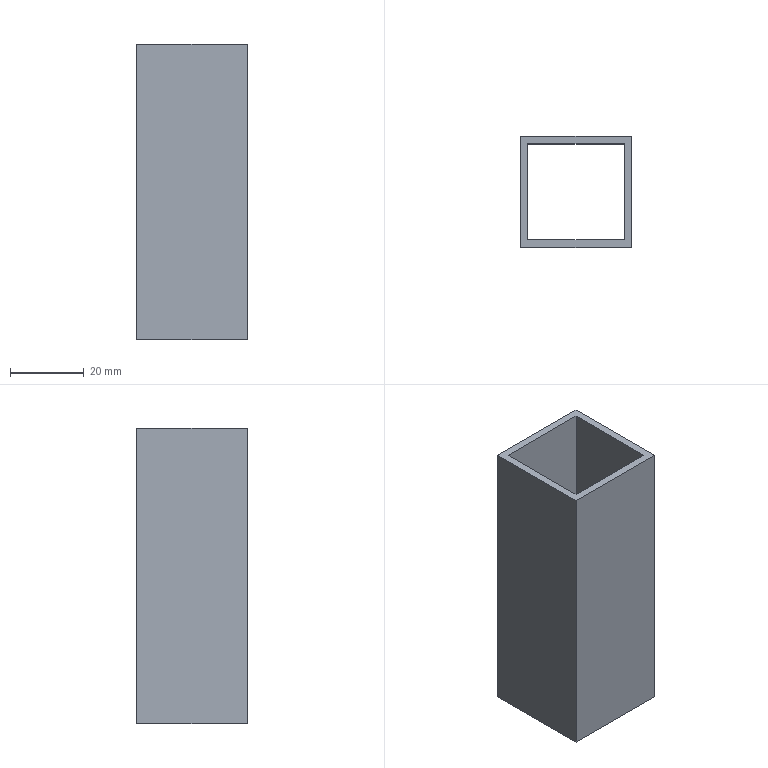Part | NX | features solid 2 | 1 solid | 10 faces | box 30 x 30 x 80 mm | volume 17920 mm3 | plane 10
STEP:
#1=CARTESIAN_POINT('',(135.,240.,-30.));
#2=VERTEX_POINT('',#1);
#3=CARTESIAN_POINT('',(105.,240.,-30.));
#4=VERTEX_POINT('',#3);
#5=CARTESIAN_POINT('',(135.,240.,-30.));
#6=DIRECTION('',(-1.,0.,0.));
#7=VECTOR('',#6,1000.);
#8=LINE('',#5,#7);
#9=EDGE_CURVE('',#2,#4,#8,.T.);
#10=ORIENTED_EDGE('',*,*,#9,.F.);
#11=CARTESIAN_POINT('',(135.,270.,-30.));
#12=VERTEX_POINT('',#11);
#13=CARTESIAN_POINT('',(135.,270.,-30.));
#14=DIRECTION('',(0.,-1.,0.));
#15=VECTOR('',#14,1000.);
#16=LINE('',#13,#15);
#17=EDGE_CURVE('',#12,#2,#16,.T.);
#18=ORIENTED_EDGE('',*,*,#17,.F.);
#19=CARTESIAN_POINT('',(105.,270.,-30.));
#20=VERTEX_POINT('',#19);
#21=CARTESIAN_POINT('',(135.,270.,-30.));
#22=DIRECTION('',(-1.,0.,0.));
#23=VECTOR('',#22,1000.);
#24=LINE('',#21,#23);
#25=EDGE_CURVE('',#12,#20,#24,.T.);
#26=ORIENTED_EDGE('',*,*,#25,.T.);
#27=CARTESIAN_POINT('',(105.,270.,-30.));
#28=DIRECTION('',(0.,-1.,0.));
#29=VECTOR('',#28,1000.);
#30=LINE('',#27,#29);
#31=EDGE_CURVE('',#20,#4,#30,.T.);
#32=ORIENTED_EDGE('',*,*,#31,.T.);
#33=EDGE_LOOP('',(#10,#18,#26,#32));
#34=FACE_BOUND('',#33,.T.);
#35=CARTESIAN_POINT('',(133.,242.,-30.));
#36=VERTEX_POINT('',#35);
#37=CARTESIAN_POINT('',(107.,242.,-30.));
#38=VERTEX_POINT('',#37);
#39=CARTESIAN_POINT('',(135.,242.,-30.));
#40=DIRECTION('',(1.,0.,0.));
#41=VECTOR('',#40,1000.);
#42=LINE('',#39,#41);
#43=EDGE_CURVE('',#36,#38,#42,.F.);
#44=ORIENTED_EDGE('',*,*,#43,.T.);
#45=CARTESIAN_POINT('',(107.,268.,-30.));
#46=VERTEX_POINT('',#45);
#47=CARTESIAN_POINT('',(107.,270.,-30.));
#48=DIRECTION('',(0.,-1.,0.));
#49=VECTOR('',#48,1000.);
#50=LINE('',#47,#49);
#51=EDGE_CURVE('',#46,#38,#50,.T.);
#52=ORIENTED_EDGE('',*,*,#51,.F.);
#53=CARTESIAN_POINT('',(133.,268.,-30.));
#54=VERTEX_POINT('',#53);
#55=CARTESIAN_POINT('',(135.,268.,-30.));
#56=DIRECTION('',(-1.,0.,0.));
#57=VECTOR('',#56,1000.);
#58=LINE('',#55,#57);
#59=EDGE_CURVE('',#54,#46,#58,.T.);
#60=ORIENTED_EDGE('',*,*,#59,.F.);
#61=CARTESIAN_POINT('',(133.,270.,-30.));
#62=DIRECTION('',(0.,1.,0.));
#63=VECTOR('',#62,1000.);
#64=LINE('',#61,#63);
#65=EDGE_CURVE('',#54,#36,#64,.F.);
#66=ORIENTED_EDGE('',*,*,#65,.T.);
#67=EDGE_LOOP('',(#44,#52,#60,#66));
#68=FACE_BOUND('',#67,.T.);
#69=CARTESIAN_POINT('',(135.,270.,-30.));
#70=DIRECTION('',(0.,0.,-1.));
#71=DIRECTION('',(1.,0.,0.));
#72=AXIS2_PLACEMENT_3D('',#69,#70,#71);
#73=PLANE('',#72);
#74=ADVANCED_FACE('',(#34,#68),#73,.F.);
#75=CARTESIAN_POINT('',(135.,240.,-110.));
#76=VERTEX_POINT('',#75);
#77=CARTESIAN_POINT('',(105.,240.,-110.));
#78=VERTEX_POINT('',#77);
#79=CARTESIAN_POINT('',(135.,240.,-110.));
#80=DIRECTION('',(1.,0.,0.));
#81=VECTOR('',#80,1000.);
#82=LINE('',#79,#81);
#83=EDGE_CURVE('',#76,#78,#82,.F.);
#84=ORIENTED_EDGE('',*,*,#83,.T.);
#85=CARTESIAN_POINT('',(105.,270.,-110.));
#86=VERTEX_POINT('',#85);
#87=CARTESIAN_POINT('',(105.,270.,-110.));
#88=DIRECTION('',(0.,-1.,0.));
#89=VECTOR('',#88,1000.);
#90=LINE('',#87,#89);
#91=EDGE_CURVE('',#86,#78,#90,.T.);
#92=ORIENTED_EDGE('',*,*,#91,.F.);
#93=CARTESIAN_POINT('',(135.,270.,-110.));
#94=VERTEX_POINT('',#93);
#95=CARTESIAN_POINT('',(135.,270.,-110.));
#96=DIRECTION('',(-1.,0.,0.));
#97=VECTOR('',#96,1000.);
#98=LINE('',#95,#97);
#99=EDGE_CURVE('',#94,#86,#98,.T.);
#100=ORIENTED_EDGE('',*,*,#99,.F.);
#101=CARTESIAN_POINT('',(135.,270.,-110.));
#102=DIRECTION('',(0.,1.,0.));
#103=VECTOR('',#102,1000.);
#104=LINE('',#101,#103);
#105=EDGE_CURVE('',#94,#76,#104,.F.);
#106=ORIENTED_EDGE('',*,*,#105,.T.);
#107=EDGE_LOOP('',(#84,#92,#100,#106));
#108=FACE_BOUND('',#107,.T.);
#109=CARTESIAN_POINT('',(133.,268.,-110.));
#110=VERTEX_POINT('',#109);
#111=CARTESIAN_POINT('',(133.,242.,-110.));
#112=VERTEX_POINT('',#111);
#113=CARTESIAN_POINT('',(133.,270.,-110.));
#114=DIRECTION('',(0.,1.,0.));
#115=VECTOR('',#114,1000.);
#116=LINE('',#113,#115);
#117=EDGE_CURVE('',#110,#112,#116,.F.);
#118=ORIENTED_EDGE('',*,*,#117,.F.);
#119=CARTESIAN_POINT('',(107.,268.,-110.));
#120=VERTEX_POINT('',#119);
#121=CARTESIAN_POINT('',(135.,268.,-110.));
#122=DIRECTION('',(-1.,0.,0.));
#123=VECTOR('',#122,1000.);
#124=LINE('',#121,#123);
#125=EDGE_CURVE('',#110,#120,#124,.T.);
#126=ORIENTED_EDGE('',*,*,#125,.T.);
#127=CARTESIAN_POINT('',(107.,242.,-110.));
#128=VERTEX_POINT('',#127);
#129=CARTESIAN_POINT('',(107.,270.,-110.));
#130=DIRECTION('',(0.,-1.,0.));
#131=VECTOR('',#130,1000.);
#132=LINE('',#129,#131);
#133=EDGE_CURVE('',#120,#128,#132,.T.);
#134=ORIENTED_EDGE('',*,*,#133,.T.);
#135=CARTESIAN_POINT('',(135.,242.,-110.));
#136=DIRECTION('',(1.,0.,0.));
#137=VECTOR('',#136,1000.);
#138=LINE('',#135,#137);
#139=EDGE_CURVE('',#112,#128,#138,.F.);
#140=ORIENTED_EDGE('',*,*,#139,.F.);
#141=EDGE_LOOP('',(#118,#126,#134,#140));
#142=FACE_BOUND('',#141,.T.);
#143=CARTESIAN_POINT('',(135.,270.,-110.));
#144=DIRECTION('',(0.,0.,-1.));
#145=DIRECTION('',(1.,0.,0.));
#146=AXIS2_PLACEMENT_3D('',#143,#144,#145);
#147=PLANE('',#146);
#148=ADVANCED_FACE('',(#108,#142),#147,.T.);
#149=CARTESIAN_POINT('',(105.,270.,-30.));
#150=DIRECTION('',(0.,0.,1.));
#151=VECTOR('',#150,1000.);
#152=LINE('',#149,#151);
#153=EDGE_CURVE('',#86,#20,#152,.T.);
#154=ORIENTED_EDGE('',*,*,#153,.T.);
#155=ORIENTED_EDGE('',*,*,#25,.F.);
#156=CARTESIAN_POINT('',(135.,270.,-30.));
#157=DIRECTION('',(0.,0.,1.));
#158=VECTOR('',#157,1000.);
#159=LINE('',#156,#158);
#160=EDGE_CURVE('',#94,#12,#159,.T.);
#161=ORIENTED_EDGE('',*,*,#160,.F.);
#162=ORIENTED_EDGE('',*,*,#99,.T.);
#163=EDGE_LOOP('',(#154,#155,#161,#162));
#164=FACE_BOUND('',#163,.T.);
#165=CARTESIAN_POINT('',(135.,270.,-30.));
#166=DIRECTION('',(0.,1.,0.));
#167=DIRECTION('',(-1.,0.,0.));
#168=AXIS2_PLACEMENT_3D('',#165,#166,#167);
#169=PLANE('',#168);
#170=ADVANCED_FACE('',(#164),#169,.T.);
#171=ORIENTED_EDGE('',*,*,#160,.T.);
#172=ORIENTED_EDGE('',*,*,#17,.T.);
#173=CARTESIAN_POINT('',(135.,240.,-30.));
#174=DIRECTION('',(0.,0.,1.));
#175=VECTOR('',#174,1000.);
#176=LINE('',#173,#175);
#177=EDGE_CURVE('',#76,#2,#176,.T.);
#178=ORIENTED_EDGE('',*,*,#177,.F.);
#179=ORIENTED_EDGE('',*,*,#105,.F.);
#180=EDGE_LOOP('',(#171,#172,#178,#179));
#181=FACE_BOUND('',#180,.T.);
#182=CARTESIAN_POINT('',(135.,270.,-30.));
#183=DIRECTION('',(-1.,0.,0.));
#184=DIRECTION('',(0.,-1.,0.));
#185=AXIS2_PLACEMENT_3D('',#182,#183,#184);
#186=PLANE('',#185);
#187=ADVANCED_FACE('',(#181),#186,.F.);
#188=ORIENTED_EDGE('',*,*,#177,.T.);
#189=ORIENTED_EDGE('',*,*,#9,.T.);
#190=CARTESIAN_POINT('',(105.,240.,-30.));
#191=DIRECTION('',(0.,0.,1.));
#192=VECTOR('',#191,1000.);
#193=LINE('',#190,#192);
#194=EDGE_CURVE('',#78,#4,#193,.T.);
#195=ORIENTED_EDGE('',*,*,#194,.F.);
#196=ORIENTED_EDGE('',*,*,#83,.F.);
#197=EDGE_LOOP('',(#188,#189,#195,#196));
#198=FACE_BOUND('',#197,.T.);
#199=CARTESIAN_POINT('',(135.,240.,-30.));
#200=DIRECTION('',(0.,1.,0.));
#201=DIRECTION('',(-1.,0.,0.));
#202=AXIS2_PLACEMENT_3D('',#199,#200,#201);
#203=PLANE('',#202);
#204=ADVANCED_FACE('',(#198),#203,.F.);
#205=ORIENTED_EDGE('',*,*,#91,.T.);
#206=ORIENTED_EDGE('',*,*,#194,.T.);
#207=ORIENTED_EDGE('',*,*,#31,.F.);
#208=ORIENTED_EDGE('',*,*,#153,.F.);
#209=EDGE_LOOP('',(#205,#206,#207,#208));
#210=FACE_BOUND('',#209,.T.);
#211=CARTESIAN_POINT('',(105.,270.,-30.));
#212=DIRECTION('',(-1.,0.,0.));
#213=DIRECTION('',(0.,-1.,0.));
#214=AXIS2_PLACEMENT_3D('',#211,#212,#213);
#215=PLANE('',#214);
#216=ADVANCED_FACE('',(#210),#215,.T.);
#217=CARTESIAN_POINT('',(107.,268.,-30.));
#218=DIRECTION('',(0.,0.,1.));
#219=VECTOR('',#218,1000.);
#220=LINE('',#217,#219);
#221=EDGE_CURVE('',#120,#46,#220,.T.);
#222=ORIENTED_EDGE('',*,*,#221,.F.);
#223=ORIENTED_EDGE('',*,*,#125,.F.);
#224=CARTESIAN_POINT('',(133.,268.,-30.));
#225=DIRECTION('',(0.,0.,-1.));
#226=VECTOR('',#225,1000.);
#227=LINE('',#224,#226);
#228=EDGE_CURVE('',#110,#54,#227,.F.);
#229=ORIENTED_EDGE('',*,*,#228,.T.);
#230=ORIENTED_EDGE('',*,*,#59,.T.);
#231=EDGE_LOOP('',(#222,#223,#229,#230));
#232=FACE_BOUND('',#231,.T.);
#233=CARTESIAN_POINT('',(135.,268.,-30.));
#234=DIRECTION('',(0.,1.,0.));
#235=DIRECTION('',(-1.,0.,0.));
#236=AXIS2_PLACEMENT_3D('',#233,#234,#235);
#237=PLANE('',#236);
#238=ADVANCED_FACE('',(#232),#237,.F.);
#239=ORIENTED_EDGE('',*,*,#228,.F.);
#240=ORIENTED_EDGE('',*,*,#117,.T.);
#241=CARTESIAN_POINT('',(133.,242.,-30.));
#242=DIRECTION('',(0.,0.,1.));
#243=VECTOR('',#242,1000.);
#244=LINE('',#241,#243);
#245=EDGE_CURVE('',#112,#36,#244,.T.);
#246=ORIENTED_EDGE('',*,*,#245,.T.);
#247=ORIENTED_EDGE('',*,*,#65,.F.);
#248=EDGE_LOOP('',(#239,#240,#246,#247));
#249=FACE_BOUND('',#248,.T.);
#250=CARTESIAN_POINT('',(133.,270.,-30.));
#251=DIRECTION('',(-1.,0.,0.));
#252=DIRECTION('',(0.,-1.,0.));
#253=AXIS2_PLACEMENT_3D('',#250,#251,#252);
#254=PLANE('',#253);
#255=ADVANCED_FACE('',(#249),#254,.T.);
#256=ORIENTED_EDGE('',*,*,#245,.F.);
#257=ORIENTED_EDGE('',*,*,#139,.T.);
#258=CARTESIAN_POINT('',(107.,242.,-30.));
#259=DIRECTION('',(0.,0.,-1.));
#260=VECTOR('',#259,1000.);
#261=LINE('',#258,#260);
#262=EDGE_CURVE('',#128,#38,#261,.F.);
#263=ORIENTED_EDGE('',*,*,#262,.T.);
#264=ORIENTED_EDGE('',*,*,#43,.F.);
#265=EDGE_LOOP('',(#256,#257,#263,#264));
#266=FACE_BOUND('',#265,.T.);
#267=CARTESIAN_POINT('',(135.,242.,-30.));
#268=DIRECTION('',(0.,1.,0.));
#269=DIRECTION('',(-1.,0.,0.));
#270=AXIS2_PLACEMENT_3D('',#267,#268,#269);
#271=PLANE('',#270);
#272=ADVANCED_FACE('',(#266),#271,.T.);
#273=ORIENTED_EDGE('',*,*,#133,.F.);
#274=ORIENTED_EDGE('',*,*,#221,.T.);
#275=ORIENTED_EDGE('',*,*,#51,.T.);
#276=ORIENTED_EDGE('',*,*,#262,.F.);
#277=EDGE_LOOP('',(#273,#274,#275,#276));
#278=FACE_BOUND('',#277,.T.);
#279=CARTESIAN_POINT('',(107.,270.,-30.));
#280=DIRECTION('',(-1.,0.,0.));
#281=DIRECTION('',(0.,-1.,0.));
#282=AXIS2_PLACEMENT_3D('',#279,#280,#281);
#283=PLANE('',#282);
#284=ADVANCED_FACE('',(#278),#283,.F.);
#285=CLOSED_SHELL('',(#74,#148,#170,#187,#204,#216,#238,#255,#272,#284));
#286=MANIFOLD_SOLID_BREP('',#285);
#287=(LENGTH_UNIT()NAMED_UNIT(*)SI_UNIT(.MILLI.,.METRE.));
#288=UNCERTAINTY_MEASURE_WITH_UNIT(LENGTH_MEASURE(0.00001),#287,'','');
#289=(NAMED_UNIT(*)PLANE_ANGLE_UNIT()SI_UNIT($,.RADIAN.));
#290=(NAMED_UNIT(*)SI_UNIT($,.STERADIAN.)SOLID_ANGLE_UNIT());
#291=(GEOMETRIC_REPRESENTATION_CONTEXT(3)GLOBAL_UNCERTAINTY_ASSIGNED_CONTEXT((#288))GLOBAL_UNIT_ASSIGNED_CONTEXT((#287,#289,#290))REPRESENTATION_CONTEXT('',''));
#292=ADVANCED_BREP_SHAPE_REPRESENTATION('',(#286),#291);